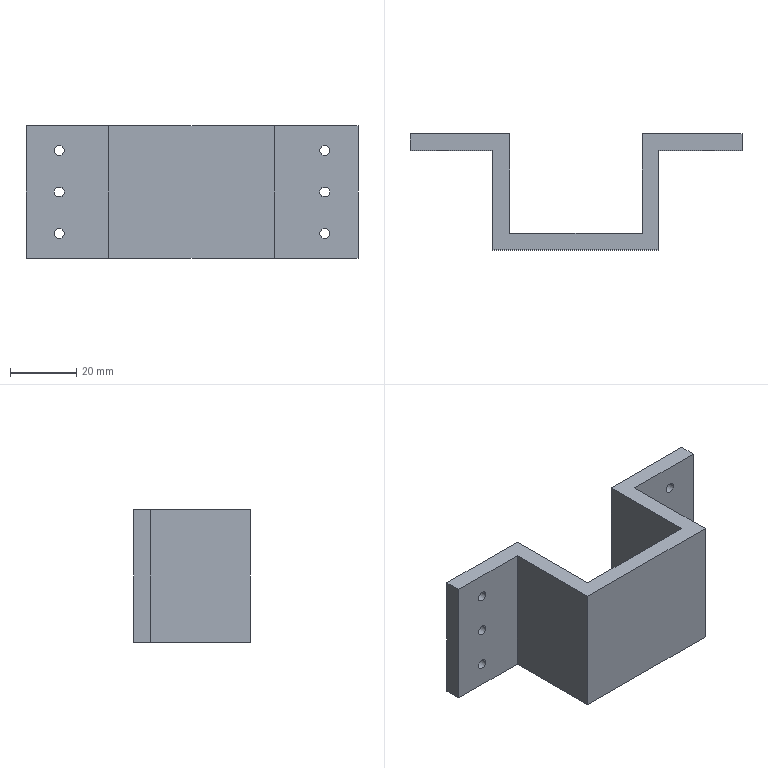Part | SolidWorks | features Extrusion 1, ICE 1 | 1 solid | 26 faces | box 100 x 35 x 40 mm | volume 31788 mm3 | plane 14 | cylinder 12 | commonest cylinder face diameters 3 x12
STEP:
#1=CARTESIAN_POINT('',(41.5,30.,7.5));
#2=VERTEX_POINT('',#1);
#3=CARTESIAN_POINT('',(38.5,30.,7.5));
#4=VERTEX_POINT('',#3);
#5=CARTESIAN_POINT('',(40.,30.,7.5));
#6=DIRECTION('',(0.,1.,0.));
#7=DIRECTION('',(-1.,0.,0.));
#8=AXIS2_PLACEMENT_3D('',#5,#6,#7);
#9=CIRCLE('',#8,1.5);
#10=EDGE_CURVE('',#2,#4,#9,.T.);
#11=ORIENTED_EDGE('',*,*,#10,.F.);
#12=CARTESIAN_POINT('',(41.5,35.,7.5));
#13=VERTEX_POINT('',#12);
#14=CARTESIAN_POINT('',(41.5,0.,7.5));
#15=DIRECTION('',(0.,1.,0.));
#16=VECTOR('',#15,1000.);
#17=LINE('',#14,#16);
#18=EDGE_CURVE('',#2,#13,#17,.T.);
#19=ORIENTED_EDGE('',*,*,#18,.T.);
#20=CARTESIAN_POINT('',(38.5,35.,7.5));
#21=VERTEX_POINT('',#20);
#22=CARTESIAN_POINT('',(40.,35.,7.5));
#23=DIRECTION('',(0.,1.,0.));
#24=DIRECTION('',(-1.,0.,0.));
#25=AXIS2_PLACEMENT_3D('',#22,#23,#24);
#26=CIRCLE('',#25,1.5);
#27=EDGE_CURVE('',#13,#21,#26,.T.);
#28=ORIENTED_EDGE('',*,*,#27,.T.);
#29=CARTESIAN_POINT('',(38.5,0.,7.5));
#30=DIRECTION('',(0.,1.,0.));
#31=VECTOR('',#30,1000.);
#32=LINE('',#29,#31);
#33=EDGE_CURVE('',#4,#21,#32,.T.);
#34=ORIENTED_EDGE('',*,*,#33,.F.);
#35=EDGE_LOOP('',(#11,#19,#28,#34));
#36=FACE_OUTER_BOUND('',#35,.T.);
#37=CARTESIAN_POINT('',(40.,0.,7.5));
#38=DIRECTION('',(0.,1.,0.));
#39=DIRECTION('',(-1.,0.,0.));
#40=AXIS2_PLACEMENT_3D('',#37,#38,#39);
#41=CYLINDRICAL_SURFACE('',#40,1.5);
#42=ADVANCED_FACE('',(#36),#41,.F.);
#43=CARTESIAN_POINT('',(41.5,30.,20.));
#44=VERTEX_POINT('',#43);
#45=CARTESIAN_POINT('',(38.5,30.,20.));
#46=VERTEX_POINT('',#45);
#47=CARTESIAN_POINT('',(40.,30.,20.));
#48=DIRECTION('',(0.,1.,0.));
#49=DIRECTION('',(-1.,0.,0.));
#50=AXIS2_PLACEMENT_3D('',#47,#48,#49);
#51=CIRCLE('',#50,1.5);
#52=EDGE_CURVE('',#44,#46,#51,.T.);
#53=ORIENTED_EDGE('',*,*,#52,.F.);
#54=CARTESIAN_POINT('',(41.5,35.,20.));
#55=VERTEX_POINT('',#54);
#56=CARTESIAN_POINT('',(41.5,0.,20.));
#57=DIRECTION('',(0.,1.,0.));
#58=VECTOR('',#57,1000.);
#59=LINE('',#56,#58);
#60=EDGE_CURVE('',#44,#55,#59,.T.);
#61=ORIENTED_EDGE('',*,*,#60,.T.);
#62=CARTESIAN_POINT('',(38.5,35.,20.));
#63=VERTEX_POINT('',#62);
#64=CARTESIAN_POINT('',(40.,35.,20.));
#65=DIRECTION('',(0.,1.,0.));
#66=DIRECTION('',(-1.,0.,0.));
#67=AXIS2_PLACEMENT_3D('',#64,#65,#66);
#68=CIRCLE('',#67,1.5);
#69=EDGE_CURVE('',#55,#63,#68,.T.);
#70=ORIENTED_EDGE('',*,*,#69,.T.);
#71=CARTESIAN_POINT('',(38.5,0.,20.));
#72=DIRECTION('',(0.,1.,0.));
#73=VECTOR('',#72,1000.);
#74=LINE('',#71,#73);
#75=EDGE_CURVE('',#46,#63,#74,.T.);
#76=ORIENTED_EDGE('',*,*,#75,.F.);
#77=EDGE_LOOP('',(#53,#61,#70,#76));
#78=FACE_OUTER_BOUND('',#77,.T.);
#79=CARTESIAN_POINT('',(40.,0.,20.));
#80=DIRECTION('',(0.,1.,0.));
#81=DIRECTION('',(-1.,0.,0.));
#82=AXIS2_PLACEMENT_3D('',#79,#80,#81);
#83=CYLINDRICAL_SURFACE('',#82,1.5);
#84=ADVANCED_FACE('',(#78),#83,.F.);
#85=CARTESIAN_POINT('',(41.5,30.,32.5));
#86=VERTEX_POINT('',#85);
#87=CARTESIAN_POINT('',(38.5,30.,32.5));
#88=VERTEX_POINT('',#87);
#89=CARTESIAN_POINT('',(40.,30.,32.5));
#90=DIRECTION('',(0.,1.,0.));
#91=DIRECTION('',(-1.,0.,0.));
#92=AXIS2_PLACEMENT_3D('',#89,#90,#91);
#93=CIRCLE('',#92,1.5);
#94=EDGE_CURVE('',#86,#88,#93,.T.);
#95=ORIENTED_EDGE('',*,*,#94,.F.);
#96=CARTESIAN_POINT('',(41.5,35.,32.5));
#97=VERTEX_POINT('',#96);
#98=CARTESIAN_POINT('',(41.5,0.,32.5));
#99=DIRECTION('',(0.,1.,0.));
#100=VECTOR('',#99,1000.);
#101=LINE('',#98,#100);
#102=EDGE_CURVE('',#86,#97,#101,.T.);
#103=ORIENTED_EDGE('',*,*,#102,.T.);
#104=CARTESIAN_POINT('',(38.5,35.,32.5));
#105=VERTEX_POINT('',#104);
#106=CARTESIAN_POINT('',(40.,35.,32.5));
#107=DIRECTION('',(0.,1.,0.));
#108=DIRECTION('',(-1.,0.,0.));
#109=AXIS2_PLACEMENT_3D('',#106,#107,#108);
#110=CIRCLE('',#109,1.5);
#111=EDGE_CURVE('',#97,#105,#110,.T.);
#112=ORIENTED_EDGE('',*,*,#111,.T.);
#113=CARTESIAN_POINT('',(38.5,0.,32.5));
#114=DIRECTION('',(0.,1.,0.));
#115=VECTOR('',#114,1000.);
#116=LINE('',#113,#115);
#117=EDGE_CURVE('',#88,#105,#116,.T.);
#118=ORIENTED_EDGE('',*,*,#117,.F.);
#119=EDGE_LOOP('',(#95,#103,#112,#118));
#120=FACE_OUTER_BOUND('',#119,.T.);
#121=CARTESIAN_POINT('',(40.,0.,32.5));
#122=DIRECTION('',(0.,1.,0.));
#123=DIRECTION('',(-1.,0.,0.));
#124=AXIS2_PLACEMENT_3D('',#121,#122,#123);
#125=CYLINDRICAL_SURFACE('',#124,1.5);
#126=ADVANCED_FACE('',(#120),#125,.F.);
#127=CARTESIAN_POINT('',(-38.5,30.,20.));
#128=VERTEX_POINT('',#127);
#129=CARTESIAN_POINT('',(-41.5,30.,20.));
#130=VERTEX_POINT('',#129);
#131=CARTESIAN_POINT('',(-40.,30.,20.));
#132=DIRECTION('',(0.,1.,0.));
#133=DIRECTION('',(-1.,0.,0.));
#134=AXIS2_PLACEMENT_3D('',#131,#132,#133);
#135=CIRCLE('',#134,1.5);
#136=EDGE_CURVE('',#128,#130,#135,.T.);
#137=ORIENTED_EDGE('',*,*,#136,.F.);
#138=CARTESIAN_POINT('',(-38.5,35.,20.));
#139=VERTEX_POINT('',#138);
#140=CARTESIAN_POINT('',(-38.5,0.,20.));
#141=DIRECTION('',(0.,1.,0.));
#142=VECTOR('',#141,1000.);
#143=LINE('',#140,#142);
#144=EDGE_CURVE('',#128,#139,#143,.T.);
#145=ORIENTED_EDGE('',*,*,#144,.T.);
#146=CARTESIAN_POINT('',(-41.5,35.,20.));
#147=VERTEX_POINT('',#146);
#148=CARTESIAN_POINT('',(-40.,35.,20.));
#149=DIRECTION('',(0.,1.,0.));
#150=DIRECTION('',(-1.,0.,0.));
#151=AXIS2_PLACEMENT_3D('',#148,#149,#150);
#152=CIRCLE('',#151,1.5);
#153=EDGE_CURVE('',#139,#147,#152,.T.);
#154=ORIENTED_EDGE('',*,*,#153,.T.);
#155=CARTESIAN_POINT('',(-41.5,0.,20.));
#156=DIRECTION('',(0.,1.,0.));
#157=VECTOR('',#156,1000.);
#158=LINE('',#155,#157);
#159=EDGE_CURVE('',#130,#147,#158,.T.);
#160=ORIENTED_EDGE('',*,*,#159,.F.);
#161=EDGE_LOOP('',(#137,#145,#154,#160));
#162=FACE_OUTER_BOUND('',#161,.T.);
#163=CARTESIAN_POINT('',(-40.,0.,20.));
#164=DIRECTION('',(0.,1.,0.));
#165=DIRECTION('',(-1.,0.,0.));
#166=AXIS2_PLACEMENT_3D('',#163,#164,#165);
#167=CYLINDRICAL_SURFACE('',#166,1.5);
#168=ADVANCED_FACE('',(#162),#167,.F.);
#169=CARTESIAN_POINT('',(-38.5,30.,32.5));
#170=VERTEX_POINT('',#169);
#171=CARTESIAN_POINT('',(-41.5,30.,32.5));
#172=VERTEX_POINT('',#171);
#173=CARTESIAN_POINT('',(-40.,30.,32.5));
#174=DIRECTION('',(0.,1.,0.));
#175=DIRECTION('',(-1.,0.,0.));
#176=AXIS2_PLACEMENT_3D('',#173,#174,#175);
#177=CIRCLE('',#176,1.5);
#178=EDGE_CURVE('',#170,#172,#177,.T.);
#179=ORIENTED_EDGE('',*,*,#178,.F.);
#180=CARTESIAN_POINT('',(-38.5,35.,32.5));
#181=VERTEX_POINT('',#180);
#182=CARTESIAN_POINT('',(-38.5,0.,32.5));
#183=DIRECTION('',(0.,1.,0.));
#184=VECTOR('',#183,1000.);
#185=LINE('',#182,#184);
#186=EDGE_CURVE('',#170,#181,#185,.T.);
#187=ORIENTED_EDGE('',*,*,#186,.T.);
#188=CARTESIAN_POINT('',(-41.5,35.,32.5));
#189=VERTEX_POINT('',#188);
#190=CARTESIAN_POINT('',(-40.,35.,32.5));
#191=DIRECTION('',(0.,1.,0.));
#192=DIRECTION('',(-1.,0.,0.));
#193=AXIS2_PLACEMENT_3D('',#190,#191,#192);
#194=CIRCLE('',#193,1.5);
#195=EDGE_CURVE('',#181,#189,#194,.T.);
#196=ORIENTED_EDGE('',*,*,#195,.T.);
#197=CARTESIAN_POINT('',(-41.5,0.,32.5));
#198=DIRECTION('',(0.,1.,0.));
#199=VECTOR('',#198,1000.);
#200=LINE('',#197,#199);
#201=EDGE_CURVE('',#172,#189,#200,.T.);
#202=ORIENTED_EDGE('',*,*,#201,.F.);
#203=EDGE_LOOP('',(#179,#187,#196,#202));
#204=FACE_OUTER_BOUND('',#203,.T.);
#205=CARTESIAN_POINT('',(-40.,0.,32.5));
#206=DIRECTION('',(0.,1.,0.));
#207=DIRECTION('',(-1.,0.,0.));
#208=AXIS2_PLACEMENT_3D('',#205,#206,#207);
#209=CYLINDRICAL_SURFACE('',#208,1.5);
#210=ADVANCED_FACE('',(#204),#209,.F.);
#211=CARTESIAN_POINT('',(-38.5,30.,7.5));
#212=VERTEX_POINT('',#211);
#213=CARTESIAN_POINT('',(-41.5,30.,7.5));
#214=VERTEX_POINT('',#213);
#215=CARTESIAN_POINT('',(-40.,30.,7.5));
#216=DIRECTION('',(0.,1.,0.));
#217=DIRECTION('',(-1.,0.,0.));
#218=AXIS2_PLACEMENT_3D('',#215,#216,#217);
#219=CIRCLE('',#218,1.5);
#220=EDGE_CURVE('',#212,#214,#219,.T.);
#221=ORIENTED_EDGE('',*,*,#220,.F.);
#222=CARTESIAN_POINT('',(-38.5,35.,7.5));
#223=VERTEX_POINT('',#222);
#224=CARTESIAN_POINT('',(-38.5,0.,7.5));
#225=DIRECTION('',(0.,1.,0.));
#226=VECTOR('',#225,1000.);
#227=LINE('',#224,#226);
#228=EDGE_CURVE('',#212,#223,#227,.T.);
#229=ORIENTED_EDGE('',*,*,#228,.T.);
#230=CARTESIAN_POINT('',(-41.5,35.,7.5));
#231=VERTEX_POINT('',#230);
#232=CARTESIAN_POINT('',(-40.,35.,7.5));
#233=DIRECTION('',(0.,1.,0.));
#234=DIRECTION('',(-1.,0.,0.));
#235=AXIS2_PLACEMENT_3D('',#232,#233,#234);
#236=CIRCLE('',#235,1.5);
#237=EDGE_CURVE('',#223,#231,#236,.T.);
#238=ORIENTED_EDGE('',*,*,#237,.T.);
#239=CARTESIAN_POINT('',(-41.5,0.,7.5));
#240=DIRECTION('',(0.,1.,0.));
#241=VECTOR('',#240,1000.);
#242=LINE('',#239,#241);
#243=EDGE_CURVE('',#214,#231,#242,.T.);
#244=ORIENTED_EDGE('',*,*,#243,.F.);
#245=EDGE_LOOP('',(#221,#229,#238,#244));
#246=FACE_OUTER_BOUND('',#245,.T.);
#247=CARTESIAN_POINT('',(-40.,0.,7.5));
#248=DIRECTION('',(0.,1.,0.));
#249=DIRECTION('',(-1.,0.,0.));
#250=AXIS2_PLACEMENT_3D('',#247,#248,#249);
#251=CYLINDRICAL_SURFACE('',#250,1.5);
#252=ADVANCED_FACE('',(#246),#251,.F.);
#253=CARTESIAN_POINT('',(25.,0.,0.));
#254=VERTEX_POINT('',#253);
#255=CARTESIAN_POINT('',(25.,30.,0.));
#256=VERTEX_POINT('',#255);
#257=CARTESIAN_POINT('',(25.,0.,0.));
#258=DIRECTION('',(0.,1.,0.));
#259=VECTOR('',#258,1000.);
#260=LINE('',#257,#259);
#261=EDGE_CURVE('',#254,#256,#260,.T.);
#262=ORIENTED_EDGE('',*,*,#261,.T.);
#263=CARTESIAN_POINT('',(25.,30.,40.));
#264=VERTEX_POINT('',#263);
#265=CARTESIAN_POINT('',(25.,30.,40.));
#266=DIRECTION('',(0.,0.,-1.));
#267=VECTOR('',#266,1000.);
#268=LINE('',#265,#267);
#269=EDGE_CURVE('',#264,#256,#268,.T.);
#270=ORIENTED_EDGE('',*,*,#269,.F.);
#271=CARTESIAN_POINT('',(25.,0.,40.));
#272=VERTEX_POINT('',#271);
#273=CARTESIAN_POINT('',(25.,0.,40.));
#274=DIRECTION('',(0.,1.,0.));
#275=VECTOR('',#274,1000.);
#276=LINE('',#273,#275);
#277=EDGE_CURVE('',#272,#264,#276,.T.);
#278=ORIENTED_EDGE('',*,*,#277,.F.);
#279=CARTESIAN_POINT('',(25.,0.,40.));
#280=DIRECTION('',(0.,0.,-1.));
#281=VECTOR('',#280,1000.);
#282=LINE('',#279,#281);
#283=EDGE_CURVE('',#272,#254,#282,.T.);
#284=ORIENTED_EDGE('',*,*,#283,.T.);
#285=EDGE_LOOP('',(#262,#270,#278,#284));
#286=FACE_OUTER_BOUND('',#285,.T.);
#287=CARTESIAN_POINT('',(25.,0.,40.));
#288=DIRECTION('',(-1.,0.,0.));
#289=DIRECTION('',(0.,0.,1.));
#290=AXIS2_PLACEMENT_3D('',#287,#288,#289);
#291=PLANE('',#290);
#292=ADVANCED_FACE('',(#286),#291,.F.);
#293=CARTESIAN_POINT('',(40.,30.,7.5));
#294=DIRECTION('',(0.,1.,0.));
#295=DIRECTION('',(-1.,0.,0.));
#296=AXIS2_PLACEMENT_3D('',#293,#294,#295);
#297=CIRCLE('',#296,1.5);
#298=EDGE_CURVE('',#4,#2,#297,.T.);
#299=ORIENTED_EDGE('',*,*,#298,.T.);
#300=ORIENTED_EDGE('',*,*,#10,.T.);
#301=EDGE_LOOP('',(#299,#300));
#302=FACE_BOUND('',#301,.T.);
#303=CARTESIAN_POINT('',(40.,30.,20.));
#304=DIRECTION('',(0.,1.,0.));
#305=DIRECTION('',(-1.,0.,0.));
#306=AXIS2_PLACEMENT_3D('',#303,#304,#305);
#307=CIRCLE('',#306,1.5);
#308=EDGE_CURVE('',#46,#44,#307,.T.);
#309=ORIENTED_EDGE('',*,*,#308,.T.);
#310=ORIENTED_EDGE('',*,*,#52,.T.);
#311=EDGE_LOOP('',(#309,#310));
#312=FACE_BOUND('',#311,.T.);
#313=CARTESIAN_POINT('',(40.,30.,32.5));
#314=DIRECTION('',(0.,1.,0.));
#315=DIRECTION('',(-1.,0.,0.));
#316=AXIS2_PLACEMENT_3D('',#313,#314,#315);
#317=CIRCLE('',#316,1.5);
#318=EDGE_CURVE('',#88,#86,#317,.T.);
#319=ORIENTED_EDGE('',*,*,#318,.T.);
#320=ORIENTED_EDGE('',*,*,#94,.T.);
#321=EDGE_LOOP('',(#319,#320));
#322=FACE_BOUND('',#321,.T.);
#323=CARTESIAN_POINT('',(50.,30.,0.));
#324=VERTEX_POINT('',#323);
#325=CARTESIAN_POINT('',(25.,30.,0.));
#326=DIRECTION('',(1.,0.,0.));
#327=VECTOR('',#326,1000.);
#328=LINE('',#325,#327);
#329=EDGE_CURVE('',#256,#324,#328,.T.);
#330=ORIENTED_EDGE('',*,*,#329,.T.);
#331=CARTESIAN_POINT('',(50.,30.,40.));
#332=VERTEX_POINT('',#331);
#333=CARTESIAN_POINT('',(50.,30.,40.));
#334=DIRECTION('',(0.,0.,-1.));
#335=VECTOR('',#334,1000.);
#336=LINE('',#333,#335);
#337=EDGE_CURVE('',#332,#324,#336,.T.);
#338=ORIENTED_EDGE('',*,*,#337,.F.);
#339=CARTESIAN_POINT('',(25.,30.,40.));
#340=DIRECTION('',(1.,0.,0.));
#341=VECTOR('',#340,1000.);
#342=LINE('',#339,#341);
#343=EDGE_CURVE('',#264,#332,#342,.T.);
#344=ORIENTED_EDGE('',*,*,#343,.F.);
#345=ORIENTED_EDGE('',*,*,#269,.T.);
#346=EDGE_LOOP('',(#330,#338,#344,#345));
#347=FACE_OUTER_BOUND('',#346,.T.);
#348=CARTESIAN_POINT('',(25.,30.,40.));
#349=DIRECTION('',(0.,1.,0.));
#350=DIRECTION('',(-1.,0.,0.));
#351=AXIS2_PLACEMENT_3D('',#348,#349,#350);
#352=PLANE('',#351);
#353=ADVANCED_FACE('',(#302,#312,#322,#347),#352,.F.);
#354=CARTESIAN_POINT('',(50.,35.,0.));
#355=VERTEX_POINT('',#354);
#356=CARTESIAN_POINT('',(50.,35.,0.));
#357=DIRECTION('',(0.,1.,0.));
#358=VECTOR('',#357,1000.);
#359=LINE('',#356,#358);
#360=EDGE_CURVE('',#324,#355,#359,.T.);
#361=ORIENTED_EDGE('',*,*,#360,.T.);
#362=CARTESIAN_POINT('',(50.,35.,40.));
#363=VERTEX_POINT('',#362);
#364=CARTESIAN_POINT('',(50.,35.,40.));
#365=DIRECTION('',(0.,0.,-1.));
#366=VECTOR('',#365,1000.);
#367=LINE('',#364,#366);
#368=EDGE_CURVE('',#363,#355,#367,.T.);
#369=ORIENTED_EDGE('',*,*,#368,.F.);
#370=CARTESIAN_POINT('',(50.,35.,40.));
#371=DIRECTION('',(0.,1.,0.));
#372=VECTOR('',#371,1000.);
#373=LINE('',#370,#372);
#374=EDGE_CURVE('',#332,#363,#373,.T.);
#375=ORIENTED_EDGE('',*,*,#374,.F.);
#376=ORIENTED_EDGE('',*,*,#337,.T.);
#377=EDGE_LOOP('',(#361,#369,#375,#376));
#378=FACE_OUTER_BOUND('',#377,.T.);
#379=CARTESIAN_POINT('',(50.,35.,40.));
#380=DIRECTION('',(-1.,0.,0.));
#381=DIRECTION('',(0.,0.,1.));
#382=AXIS2_PLACEMENT_3D('',#379,#380,#381);
#383=PLANE('',#382);
#384=ADVANCED_FACE('',(#378),#383,.F.);
#385=CARTESIAN_POINT('',(40.,35.,7.5));
#386=DIRECTION('',(0.,1.,0.));
#387=DIRECTION('',(-1.,0.,0.));
#388=AXIS2_PLACEMENT_3D('',#385,#386,#387);
#389=CIRCLE('',#388,1.5);
#390=EDGE_CURVE('',#21,#13,#389,.T.);
#391=ORIENTED_EDGE('',*,*,#390,.F.);
#392=ORIENTED_EDGE('',*,*,#27,.F.);
#393=EDGE_LOOP('',(#391,#392));
#394=FACE_BOUND('',#393,.T.);
#395=CARTESIAN_POINT('',(40.,35.,20.));
#396=DIRECTION('',(0.,1.,0.));
#397=DIRECTION('',(-1.,0.,0.));
#398=AXIS2_PLACEMENT_3D('',#395,#396,#397);
#399=CIRCLE('',#398,1.5);
#400=EDGE_CURVE('',#63,#55,#399,.T.);
#401=ORIENTED_EDGE('',*,*,#400,.F.);
#402=ORIENTED_EDGE('',*,*,#69,.F.);
#403=EDGE_LOOP('',(#401,#402));
#404=FACE_BOUND('',#403,.T.);
#405=CARTESIAN_POINT('',(40.,35.,32.5));
#406=DIRECTION('',(0.,1.,0.));
#407=DIRECTION('',(-1.,0.,0.));
#408=AXIS2_PLACEMENT_3D('',#405,#406,#407);
#409=CIRCLE('',#408,1.5);
#410=EDGE_CURVE('',#105,#97,#409,.T.);
#411=ORIENTED_EDGE('',*,*,#410,.F.);
#412=ORIENTED_EDGE('',*,*,#111,.F.);
#413=EDGE_LOOP('',(#411,#412));
#414=FACE_BOUND('',#413,.T.);
#415=CARTESIAN_POINT('',(20.,35.,0.));
#416=VERTEX_POINT('',#415);
#417=CARTESIAN_POINT('',(20.,35.,0.));
#418=DIRECTION('',(-1.,0.,0.));
#419=VECTOR('',#418,1000.);
#420=LINE('',#417,#419);
#421=EDGE_CURVE('',#355,#416,#420,.T.);
#422=ORIENTED_EDGE('',*,*,#421,.T.);
#423=CARTESIAN_POINT('',(20.,35.,40.));
#424=VERTEX_POINT('',#423);
#425=CARTESIAN_POINT('',(20.,35.,40.));
#426=DIRECTION('',(0.,0.,-1.));
#427=VECTOR('',#426,1000.);
#428=LINE('',#425,#427);
#429=EDGE_CURVE('',#424,#416,#428,.T.);
#430=ORIENTED_EDGE('',*,*,#429,.F.);
#431=CARTESIAN_POINT('',(20.,35.,40.));
#432=DIRECTION('',(-1.,0.,0.));
#433=VECTOR('',#432,1000.);
#434=LINE('',#431,#433);
#435=EDGE_CURVE('',#363,#424,#434,.T.);
#436=ORIENTED_EDGE('',*,*,#435,.F.);
#437=ORIENTED_EDGE('',*,*,#368,.T.);
#438=EDGE_LOOP('',(#422,#430,#436,#437));
#439=FACE_OUTER_BOUND('',#438,.T.);
#440=CARTESIAN_POINT('',(20.,35.,40.));
#441=DIRECTION('',(0.,-1.,0.));
#442=DIRECTION('',(1.,0.,0.));
#443=AXIS2_PLACEMENT_3D('',#440,#441,#442);
#444=PLANE('',#443);
#445=ADVANCED_FACE('',(#394,#404,#414,#439),#444,.F.);
#446=CARTESIAN_POINT('',(20.,5.,0.));
#447=VERTEX_POINT('',#446);
#448=CARTESIAN_POINT('',(20.,5.,0.));
#449=DIRECTION('',(0.,-1.,0.));
#450=VECTOR('',#449,1000.);
#451=LINE('',#448,#450);
#452=EDGE_CURVE('',#416,#447,#451,.T.);
#453=ORIENTED_EDGE('',*,*,#452,.T.);
#454=CARTESIAN_POINT('',(20.,5.,40.));
#455=VERTEX_POINT('',#454);
#456=CARTESIAN_POINT('',(20.,5.,40.));
#457=DIRECTION('',(0.,0.,-1.));
#458=VECTOR('',#457,1000.);
#459=LINE('',#456,#458);
#460=EDGE_CURVE('',#455,#447,#459,.T.);
#461=ORIENTED_EDGE('',*,*,#460,.F.);
#462=CARTESIAN_POINT('',(20.,5.,40.));
#463=DIRECTION('',(0.,-1.,0.));
#464=VECTOR('',#463,1000.);
#465=LINE('',#462,#464);
#466=EDGE_CURVE('',#424,#455,#465,.T.);
#467=ORIENTED_EDGE('',*,*,#466,.F.);
#468=ORIENTED_EDGE('',*,*,#429,.T.);
#469=EDGE_LOOP('',(#453,#461,#467,#468));
#470=FACE_OUTER_BOUND('',#469,.T.);
#471=CARTESIAN_POINT('',(20.,5.,40.));
#472=DIRECTION('',(1.,0.,0.));
#473=DIRECTION('',(0.,0.,-1.));
#474=AXIS2_PLACEMENT_3D('',#471,#472,#473);
#475=PLANE('',#474);
#476=ADVANCED_FACE('',(#470),#475,.F.);
#477=CARTESIAN_POINT('',(-20.,5.,0.));
#478=VERTEX_POINT('',#477);
#479=CARTESIAN_POINT('',(0.,5.,0.));
#480=DIRECTION('',(-1.,0.,0.));
#481=VECTOR('',#480,1000.);
#482=LINE('',#479,#481);
#483=EDGE_CURVE('',#447,#478,#482,.T.);
#484=ORIENTED_EDGE('',*,*,#483,.T.);
#485=CARTESIAN_POINT('',(-20.,5.,40.));
#486=VERTEX_POINT('',#485);
#487=CARTESIAN_POINT('',(-20.,5.,40.));
#488=DIRECTION('',(0.,0.,-1.));
#489=VECTOR('',#488,1000.);
#490=LINE('',#487,#489);
#491=EDGE_CURVE('',#486,#478,#490,.T.);
#492=ORIENTED_EDGE('',*,*,#491,.F.);
#493=CARTESIAN_POINT('',(0.,5.,40.));
#494=DIRECTION('',(-1.,0.,0.));
#495=VECTOR('',#494,1000.);
#496=LINE('',#493,#495);
#497=EDGE_CURVE('',#455,#486,#496,.T.);
#498=ORIENTED_EDGE('',*,*,#497,.F.);
#499=ORIENTED_EDGE('',*,*,#460,.T.);
#500=EDGE_LOOP('',(#484,#492,#498,#499));
#501=FACE_OUTER_BOUND('',#500,.T.);
#502=CARTESIAN_POINT('',(0.,5.,40.));
#503=DIRECTION('',(0.,-1.,0.));
#504=DIRECTION('',(1.,0.,0.));
#505=AXIS2_PLACEMENT_3D('',#502,#503,#504);
#506=PLANE('',#505);
#507=ADVANCED_FACE('',(#501),#506,.F.);
#508=CARTESIAN_POINT('',(-20.,35.,0.));
#509=VERTEX_POINT('',#508);
#510=CARTESIAN_POINT('',(-20.,5.,0.));
#511=DIRECTION('',(0.,1.,0.));
#512=VECTOR('',#511,1000.);
#513=LINE('',#510,#512);
#514=EDGE_CURVE('',#478,#509,#513,.T.);
#515=ORIENTED_EDGE('',*,*,#514,.T.);
#516=CARTESIAN_POINT('',(-20.,35.,40.));
#517=VERTEX_POINT('',#516);
#518=CARTESIAN_POINT('',(-20.,35.,40.));
#519=DIRECTION('',(0.,0.,-1.));
#520=VECTOR('',#519,1000.);
#521=LINE('',#518,#520);
#522=EDGE_CURVE('',#517,#509,#521,.T.);
#523=ORIENTED_EDGE('',*,*,#522,.F.);
#524=CARTESIAN_POINT('',(-20.,5.,40.));
#525=DIRECTION('',(0.,1.,0.));
#526=VECTOR('',#525,1000.);
#527=LINE('',#524,#526);
#528=EDGE_CURVE('',#486,#517,#527,.T.);
#529=ORIENTED_EDGE('',*,*,#528,.F.);
#530=ORIENTED_EDGE('',*,*,#491,.T.);
#531=EDGE_LOOP('',(#515,#523,#529,#530));
#532=FACE_OUTER_BOUND('',#531,.T.);
#533=CARTESIAN_POINT('',(-20.,5.,40.));
#534=DIRECTION('',(-1.,0.,0.));
#535=DIRECTION('',(0.,0.,1.));
#536=AXIS2_PLACEMENT_3D('',#533,#534,#535);
#537=PLANE('',#536);
#538=ADVANCED_FACE('',(#532),#537,.F.);
#539=CARTESIAN_POINT('',(-40.,35.,20.));
#540=DIRECTION('',(0.,1.,0.));
#541=DIRECTION('',(-1.,0.,0.));
#542=AXIS2_PLACEMENT_3D('',#539,#540,#541);
#543=CIRCLE('',#542,1.5);
#544=EDGE_CURVE('',#147,#139,#543,.T.);
#545=ORIENTED_EDGE('',*,*,#544,.F.);
#546=ORIENTED_EDGE('',*,*,#153,.F.);
#547=EDGE_LOOP('',(#545,#546));
#548=FACE_BOUND('',#547,.T.);
#549=CARTESIAN_POINT('',(-40.,35.,32.5));
#550=DIRECTION('',(0.,1.,0.));
#551=DIRECTION('',(-1.,0.,0.));
#552=AXIS2_PLACEMENT_3D('',#549,#550,#551);
#553=CIRCLE('',#552,1.5);
#554=EDGE_CURVE('',#189,#181,#553,.T.);
#555=ORIENTED_EDGE('',*,*,#554,.F.);
#556=ORIENTED_EDGE('',*,*,#195,.F.);
#557=EDGE_LOOP('',(#555,#556));
#558=FACE_BOUND('',#557,.T.);
#559=CARTESIAN_POINT('',(-40.,35.,7.5));
#560=DIRECTION('',(0.,1.,0.));
#561=DIRECTION('',(-1.,0.,0.));
#562=AXIS2_PLACEMENT_3D('',#559,#560,#561);
#563=CIRCLE('',#562,1.5);
#564=EDGE_CURVE('',#231,#223,#563,.T.);
#565=ORIENTED_EDGE('',*,*,#564,.F.);
#566=ORIENTED_EDGE('',*,*,#237,.F.);
#567=EDGE_LOOP('',(#565,#566));
#568=FACE_BOUND('',#567,.T.);
#569=CARTESIAN_POINT('',(-50.,35.,0.));
#570=VERTEX_POINT('',#569);
#571=CARTESIAN_POINT('',(-20.,35.,0.));
#572=DIRECTION('',(-1.,0.,0.));
#573=VECTOR('',#572,1000.);
#574=LINE('',#571,#573);
#575=EDGE_CURVE('',#509,#570,#574,.T.);
#576=ORIENTED_EDGE('',*,*,#575,.T.);
#577=CARTESIAN_POINT('',(-50.,35.,40.));
#578=VERTEX_POINT('',#577);
#579=CARTESIAN_POINT('',(-50.,35.,40.));
#580=DIRECTION('',(0.,0.,-1.));
#581=VECTOR('',#580,1000.);
#582=LINE('',#579,#581);
#583=EDGE_CURVE('',#578,#570,#582,.T.);
#584=ORIENTED_EDGE('',*,*,#583,.F.);
#585=CARTESIAN_POINT('',(-20.,35.,40.));
#586=DIRECTION('',(-1.,0.,0.));
#587=VECTOR('',#586,1000.);
#588=LINE('',#585,#587);
#589=EDGE_CURVE('',#517,#578,#588,.T.);
#590=ORIENTED_EDGE('',*,*,#589,.F.);
#591=ORIENTED_EDGE('',*,*,#522,.T.);
#592=EDGE_LOOP('',(#576,#584,#590,#591));
#593=FACE_OUTER_BOUND('',#592,.T.);
#594=CARTESIAN_POINT('',(-20.,35.,40.));
#595=DIRECTION('',(0.,-1.,0.));
#596=DIRECTION('',(1.,0.,0.));
#597=AXIS2_PLACEMENT_3D('',#594,#595,#596);
#598=PLANE('',#597);
#599=ADVANCED_FACE('',(#548,#558,#568,#593),#598,.F.);
#600=CARTESIAN_POINT('',(-50.,30.,0.));
#601=VERTEX_POINT('',#600);
#602=CARTESIAN_POINT('',(-50.,35.,0.));
#603=DIRECTION('',(0.,-1.,0.));
#604=VECTOR('',#603,1000.);
#605=LINE('',#602,#604);
#606=EDGE_CURVE('',#570,#601,#605,.T.);
#607=ORIENTED_EDGE('',*,*,#606,.T.);
#608=CARTESIAN_POINT('',(-50.,30.,40.));
#609=VERTEX_POINT('',#608);
#610=CARTESIAN_POINT('',(-50.,30.,40.));
#611=DIRECTION('',(0.,0.,-1.));
#612=VECTOR('',#611,1000.);
#613=LINE('',#610,#612);
#614=EDGE_CURVE('',#609,#601,#613,.T.);
#615=ORIENTED_EDGE('',*,*,#614,.F.);
#616=CARTESIAN_POINT('',(-50.,35.,40.));
#617=DIRECTION('',(0.,-1.,0.));
#618=VECTOR('',#617,1000.);
#619=LINE('',#616,#618);
#620=EDGE_CURVE('',#578,#609,#619,.T.);
#621=ORIENTED_EDGE('',*,*,#620,.F.);
#622=ORIENTED_EDGE('',*,*,#583,.T.);
#623=EDGE_LOOP('',(#607,#615,#621,#622));
#624=FACE_OUTER_BOUND('',#623,.T.);
#625=CARTESIAN_POINT('',(-50.,35.,40.));
#626=DIRECTION('',(1.,0.,0.));
#627=DIRECTION('',(0.,0.,-1.));
#628=AXIS2_PLACEMENT_3D('',#625,#626,#627);
#629=PLANE('',#628);
#630=ADVANCED_FACE('',(#624),#629,.F.);
#631=CARTESIAN_POINT('',(-40.,30.,20.));
#632=DIRECTION('',(0.,1.,0.));
#633=DIRECTION('',(-1.,0.,0.));
#634=AXIS2_PLACEMENT_3D('',#631,#632,#633);
#635=CIRCLE('',#634,1.5);
#636=EDGE_CURVE('',#130,#128,#635,.T.);
#637=ORIENTED_EDGE('',*,*,#636,.T.);
#638=ORIENTED_EDGE('',*,*,#136,.T.);
#639=EDGE_LOOP('',(#637,#638));
#640=FACE_BOUND('',#639,.T.);
#641=CARTESIAN_POINT('',(-40.,30.,32.5));
#642=DIRECTION('',(0.,1.,0.));
#643=DIRECTION('',(-1.,0.,0.));
#644=AXIS2_PLACEMENT_3D('',#641,#642,#643);
#645=CIRCLE('',#644,1.5);
#646=EDGE_CURVE('',#172,#170,#645,.T.);
#647=ORIENTED_EDGE('',*,*,#646,.T.);
#648=ORIENTED_EDGE('',*,*,#178,.T.);
#649=EDGE_LOOP('',(#647,#648));
#650=FACE_BOUND('',#649,.T.);
#651=CARTESIAN_POINT('',(-40.,30.,7.5));
#652=DIRECTION('',(0.,1.,0.));
#653=DIRECTION('',(-1.,0.,0.));
#654=AXIS2_PLACEMENT_3D('',#651,#652,#653);
#655=CIRCLE('',#654,1.5);
#656=EDGE_CURVE('',#214,#212,#655,.T.);
#657=ORIENTED_EDGE('',*,*,#656,.T.);
#658=ORIENTED_EDGE('',*,*,#220,.T.);
#659=EDGE_LOOP('',(#657,#658));
#660=FACE_BOUND('',#659,.T.);
#661=CARTESIAN_POINT('',(-25.,30.,0.));
#662=VERTEX_POINT('',#661);
#663=CARTESIAN_POINT('',(-25.,30.,0.));
#664=DIRECTION('',(1.,0.,0.));
#665=VECTOR('',#664,1000.);
#666=LINE('',#663,#665);
#667=EDGE_CURVE('',#601,#662,#666,.T.);
#668=ORIENTED_EDGE('',*,*,#667,.T.);
#669=CARTESIAN_POINT('',(-25.,30.,40.));
#670=VERTEX_POINT('',#669);
#671=CARTESIAN_POINT('',(-25.,30.,40.));
#672=DIRECTION('',(0.,0.,-1.));
#673=VECTOR('',#672,1000.);
#674=LINE('',#671,#673);
#675=EDGE_CURVE('',#670,#662,#674,.T.);
#676=ORIENTED_EDGE('',*,*,#675,.F.);
#677=CARTESIAN_POINT('',(-25.,30.,40.));
#678=DIRECTION('',(1.,0.,0.));
#679=VECTOR('',#678,1000.);
#680=LINE('',#677,#679);
#681=EDGE_CURVE('',#609,#670,#680,.T.);
#682=ORIENTED_EDGE('',*,*,#681,.F.);
#683=ORIENTED_EDGE('',*,*,#614,.T.);
#684=EDGE_LOOP('',(#668,#676,#682,#683));
#685=FACE_OUTER_BOUND('',#684,.T.);
#686=CARTESIAN_POINT('',(-25.,30.,40.));
#687=DIRECTION('',(0.,1.,0.));
#688=DIRECTION('',(-1.,0.,0.));
#689=AXIS2_PLACEMENT_3D('',#686,#687,#688);
#690=PLANE('',#689);
#691=ADVANCED_FACE('',(#640,#650,#660,#685),#690,.F.);
#692=CARTESIAN_POINT('',(-25.,0.,0.));
#693=VERTEX_POINT('',#692);
#694=CARTESIAN_POINT('',(-25.,0.,0.));
#695=DIRECTION('',(0.,-1.,0.));
#696=VECTOR('',#695,1000.);
#697=LINE('',#694,#696);
#698=EDGE_CURVE('',#662,#693,#697,.T.);
#699=ORIENTED_EDGE('',*,*,#698,.T.);
#700=CARTESIAN_POINT('',(-25.,0.,40.));
#701=VERTEX_POINT('',#700);
#702=CARTESIAN_POINT('',(-25.,0.,40.));
#703=DIRECTION('',(0.,0.,-1.));
#704=VECTOR('',#703,1000.);
#705=LINE('',#702,#704);
#706=EDGE_CURVE('',#701,#693,#705,.T.);
#707=ORIENTED_EDGE('',*,*,#706,.F.);
#708=CARTESIAN_POINT('',(-25.,0.,40.));
#709=DIRECTION('',(0.,-1.,0.));
#710=VECTOR('',#709,1000.);
#711=LINE('',#708,#710);
#712=EDGE_CURVE('',#670,#701,#711,.T.);
#713=ORIENTED_EDGE('',*,*,#712,.F.);
#714=ORIENTED_EDGE('',*,*,#675,.T.);
#715=EDGE_LOOP('',(#699,#707,#713,#714));
#716=FACE_OUTER_BOUND('',#715,.T.);
#717=CARTESIAN_POINT('',(-25.,0.,40.));
#718=DIRECTION('',(1.,0.,0.));
#719=DIRECTION('',(0.,0.,-1.));
#720=AXIS2_PLACEMENT_3D('',#717,#718,#719);
#721=PLANE('',#720);
#722=ADVANCED_FACE('',(#716),#721,.F.);
#723=CARTESIAN_POINT('',(0.,0.,0.));
#724=DIRECTION('',(1.,0.,0.));
#725=VECTOR('',#724,1000.);
#726=LINE('',#723,#725);
#727=EDGE_CURVE('',#693,#254,#726,.T.);
#728=ORIENTED_EDGE('',*,*,#727,.T.);
#729=ORIENTED_EDGE('',*,*,#283,.F.);
#730=CARTESIAN_POINT('',(0.,0.,40.));
#731=DIRECTION('',(1.,0.,0.));
#732=VECTOR('',#731,1000.);
#733=LINE('',#730,#732);
#734=EDGE_CURVE('',#701,#272,#733,.T.);
#735=ORIENTED_EDGE('',*,*,#734,.F.);
#736=ORIENTED_EDGE('',*,*,#706,.T.);
#737=EDGE_LOOP('',(#728,#729,#735,#736));
#738=FACE_OUTER_BOUND('',#737,.T.);
#739=CARTESIAN_POINT('',(0.,0.,40.));
#740=DIRECTION('',(0.,1.,0.));
#741=DIRECTION('',(-1.,0.,0.));
#742=AXIS2_PLACEMENT_3D('',#739,#740,#741);
#743=PLANE('',#742);
#744=ADVANCED_FACE('',(#738),#743,.F.);
#745=ORIENTED_EDGE('',*,*,#734,.T.);
#746=ORIENTED_EDGE('',*,*,#277,.T.);
#747=ORIENTED_EDGE('',*,*,#343,.T.);
#748=ORIENTED_EDGE('',*,*,#374,.T.);
#749=ORIENTED_EDGE('',*,*,#435,.T.);
#750=ORIENTED_EDGE('',*,*,#466,.T.);
#751=ORIENTED_EDGE('',*,*,#497,.T.);
#752=ORIENTED_EDGE('',*,*,#528,.T.);
#753=ORIENTED_EDGE('',*,*,#589,.T.);
#754=ORIENTED_EDGE('',*,*,#620,.T.);
#755=ORIENTED_EDGE('',*,*,#681,.T.);
#756=ORIENTED_EDGE('',*,*,#712,.T.);
#757=EDGE_LOOP('',(#745,#746,#747,#748,#749,#750,#751,#752,#753,#754,#755,#756));
#758=FACE_OUTER_BOUND('',#757,.T.);
#759=CARTESIAN_POINT('',(0.,0.,40.));
#760=DIRECTION('',(0.,0.,1.));
#761=DIRECTION('',(1.,0.,0.));
#762=AXIS2_PLACEMENT_3D('',#759,#760,#761);
#763=PLANE('',#762);
#764=ADVANCED_FACE('',(#758),#763,.T.);
#765=ORIENTED_EDGE('',*,*,#261,.F.);
#766=ORIENTED_EDGE('',*,*,#727,.F.);
#767=ORIENTED_EDGE('',*,*,#698,.F.);
#768=ORIENTED_EDGE('',*,*,#667,.F.);
#769=ORIENTED_EDGE('',*,*,#606,.F.);
#770=ORIENTED_EDGE('',*,*,#575,.F.);
#771=ORIENTED_EDGE('',*,*,#514,.F.);
#772=ORIENTED_EDGE('',*,*,#483,.F.);
#773=ORIENTED_EDGE('',*,*,#452,.F.);
#774=ORIENTED_EDGE('',*,*,#421,.F.);
#775=ORIENTED_EDGE('',*,*,#360,.F.);
#776=ORIENTED_EDGE('',*,*,#329,.F.);
#777=EDGE_LOOP('',(#765,#766,#767,#768,#769,#770,#771,#772,#773,#774,#775,#776));
#778=FACE_OUTER_BOUND('',#777,.T.);
#779=CARTESIAN_POINT('',(0.,0.,0.));
#780=DIRECTION('',(0.,0.,1.));
#781=DIRECTION('',(1.,0.,0.));
#782=AXIS2_PLACEMENT_3D('',#779,#780,#781);
#783=PLANE('',#782);
#784=ADVANCED_FACE('',(#778),#783,.F.);
#785=ORIENTED_EDGE('',*,*,#228,.F.);
#786=ORIENTED_EDGE('',*,*,#656,.F.);
#787=ORIENTED_EDGE('',*,*,#243,.T.);
#788=ORIENTED_EDGE('',*,*,#564,.T.);
#789=EDGE_LOOP('',(#785,#786,#787,#788));
#790=FACE_OUTER_BOUND('',#789,.T.);
#791=CARTESIAN_POINT('',(-40.,0.,7.5));
#792=DIRECTION('',(0.,1.,0.));
#793=DIRECTION('',(-1.,0.,0.));
#794=AXIS2_PLACEMENT_3D('',#791,#792,#793);
#795=CYLINDRICAL_SURFACE('',#794,1.5);
#796=ADVANCED_FACE('',(#790),#795,.F.);
#797=ORIENTED_EDGE('',*,*,#186,.F.);
#798=ORIENTED_EDGE('',*,*,#646,.F.);
#799=ORIENTED_EDGE('',*,*,#201,.T.);
#800=ORIENTED_EDGE('',*,*,#554,.T.);
#801=EDGE_LOOP('',(#797,#798,#799,#800));
#802=FACE_OUTER_BOUND('',#801,.T.);
#803=CARTESIAN_POINT('',(-40.,0.,32.5));
#804=DIRECTION('',(0.,1.,0.));
#805=DIRECTION('',(-1.,0.,0.));
#806=AXIS2_PLACEMENT_3D('',#803,#804,#805);
#807=CYLINDRICAL_SURFACE('',#806,1.5);
#808=ADVANCED_FACE('',(#802),#807,.F.);
#809=ORIENTED_EDGE('',*,*,#144,.F.);
#810=ORIENTED_EDGE('',*,*,#636,.F.);
#811=ORIENTED_EDGE('',*,*,#159,.T.);
#812=ORIENTED_EDGE('',*,*,#544,.T.);
#813=EDGE_LOOP('',(#809,#810,#811,#812));
#814=FACE_OUTER_BOUND('',#813,.T.);
#815=CARTESIAN_POINT('',(-40.,0.,20.));
#816=DIRECTION('',(0.,1.,0.));
#817=DIRECTION('',(-1.,0.,0.));
#818=AXIS2_PLACEMENT_3D('',#815,#816,#817);
#819=CYLINDRICAL_SURFACE('',#818,1.5);
#820=ADVANCED_FACE('',(#814),#819,.F.);
#821=ORIENTED_EDGE('',*,*,#102,.F.);
#822=ORIENTED_EDGE('',*,*,#318,.F.);
#823=ORIENTED_EDGE('',*,*,#117,.T.);
#824=ORIENTED_EDGE('',*,*,#410,.T.);
#825=EDGE_LOOP('',(#821,#822,#823,#824));
#826=FACE_OUTER_BOUND('',#825,.T.);
#827=CARTESIAN_POINT('',(40.,0.,32.5));
#828=DIRECTION('',(0.,1.,0.));
#829=DIRECTION('',(-1.,0.,0.));
#830=AXIS2_PLACEMENT_3D('',#827,#828,#829);
#831=CYLINDRICAL_SURFACE('',#830,1.5);
#832=ADVANCED_FACE('',(#826),#831,.F.);
#833=ORIENTED_EDGE('',*,*,#60,.F.);
#834=ORIENTED_EDGE('',*,*,#308,.F.);
#835=ORIENTED_EDGE('',*,*,#75,.T.);
#836=ORIENTED_EDGE('',*,*,#400,.T.);
#837=EDGE_LOOP('',(#833,#834,#835,#836));
#838=FACE_OUTER_BOUND('',#837,.T.);
#839=CARTESIAN_POINT('',(40.,0.,20.));
#840=DIRECTION('',(0.,1.,0.));
#841=DIRECTION('',(-1.,0.,0.));
#842=AXIS2_PLACEMENT_3D('',#839,#840,#841);
#843=CYLINDRICAL_SURFACE('',#842,1.5);
#844=ADVANCED_FACE('',(#838),#843,.F.);
#845=ORIENTED_EDGE('',*,*,#18,.F.);
#846=ORIENTED_EDGE('',*,*,#298,.F.);
#847=ORIENTED_EDGE('',*,*,#33,.T.);
#848=ORIENTED_EDGE('',*,*,#390,.T.);
#849=EDGE_LOOP('',(#845,#846,#847,#848));
#850=FACE_OUTER_BOUND('',#849,.T.);
#851=CARTESIAN_POINT('',(40.,0.,7.5));
#852=DIRECTION('',(0.,1.,0.));
#853=DIRECTION('',(-1.,0.,0.));
#854=AXIS2_PLACEMENT_3D('',#851,#852,#853);
#855=CYLINDRICAL_SURFACE('',#854,1.5);
#856=ADVANCED_FACE('',(#850),#855,.F.);
#857=CLOSED_SHELL('',(#42,#84,#126,#168,#210,#252,#292,#353,#384,#445,#476,#507,#538,#599,#630,#691,#722,#744,#764,#784,#796,#808,#820,#832,#844,#856));
#858=MANIFOLD_SOLID_BREP('',#857);
#859=CARTESIAN_POINT('',(0.,0.,0.));
#860=DIRECTION('',(0.,0.,1.));
#861=DIRECTION('',(1.,0.,0.));
#862=AXIS2_PLACEMENT_3D('',#859,#860,#861);
#863=(LENGTH_UNIT()NAMED_UNIT(*)SI_UNIT(.MILLI.,.METRE.));
#864=UNCERTAINTY_MEASURE_WITH_UNIT(LENGTH_MEASURE(0.00001),#863,'','');
#865=(NAMED_UNIT(*)PLANE_ANGLE_UNIT()SI_UNIT($,.RADIAN.));
#866=(NAMED_UNIT(*)SI_UNIT($,.STERADIAN.)SOLID_ANGLE_UNIT());
#867=(GEOMETRIC_REPRESENTATION_CONTEXT(3)GLOBAL_UNCERTAINTY_ASSIGNED_CONTEXT((#864))GLOBAL_UNIT_ASSIGNED_CONTEXT((#863,#865,#866))REPRESENTATION_CONTEXT('',''));
#868=ADVANCED_BREP_SHAPE_REPRESENTATION('',(#858,#862),#867);